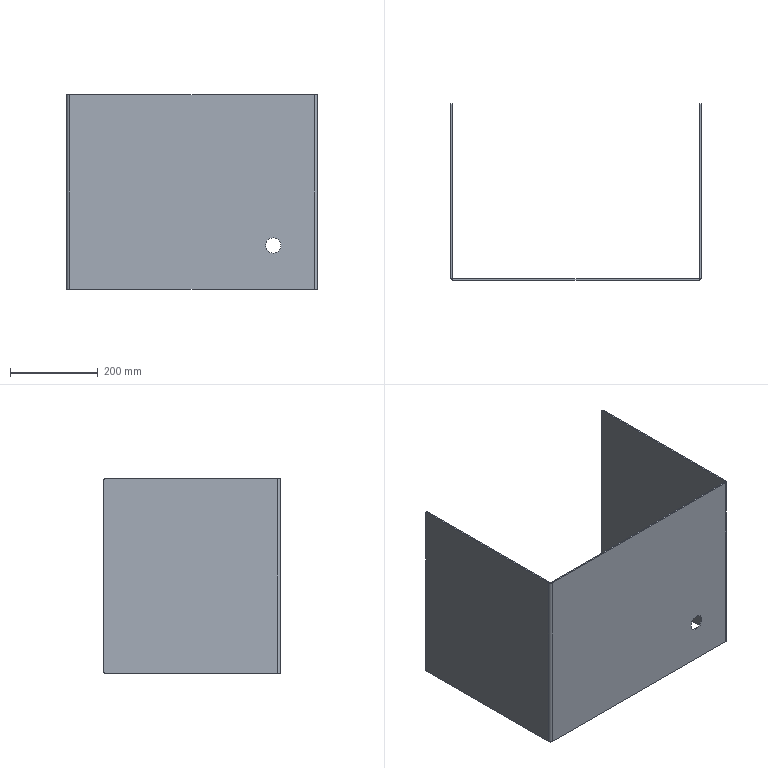Part | SolidWorks | features ICE 2, FlatPattern 1, SMBaseFlange 1, SheetMetal 1 | 1 solid | 28 faces | box 571 x 403 x 444 mm | volume 1818117 mm3 | plane 18 | cylinder 10 | commonest cylinder face diameters 6 x6 12 x2 35 x2
STEP:
#1=CARTESIAN_POINT('',(471.,3.,82.5));
#2=VERTEX_POINT('',#1);
#3=CARTESIAN_POINT('',(471.,3.,117.5));
#4=VERTEX_POINT('',#3);
#5=CARTESIAN_POINT('',(471.,3.,100.));
#6=DIRECTION('',(0.,1.,0.));
#7=DIRECTION('',(0.,0.,1.));
#8=AXIS2_PLACEMENT_3D('',#5,#6,#7);
#9=CIRCLE('',#8,17.5);
#10=EDGE_CURVE('',#2,#4,#9,.T.);
#11=ORIENTED_EDGE('',*,*,#10,.T.);
#12=CARTESIAN_POINT('',(471.,0.,117.5));
#13=VERTEX_POINT('',#12);
#14=CARTESIAN_POINT('',(471.,10.,117.5));
#15=DIRECTION('',(0.,-1.,0.));
#16=VECTOR('',#15,1000.);
#17=LINE('',#14,#16);
#18=EDGE_CURVE('',#4,#13,#17,.T.);
#19=ORIENTED_EDGE('',*,*,#18,.T.);
#20=CARTESIAN_POINT('',(471.,0.,82.5));
#21=VERTEX_POINT('',#20);
#22=CARTESIAN_POINT('',(471.,0.,100.));
#23=DIRECTION('',(0.,-1.,0.));
#24=DIRECTION('',(0.,0.,-1.));
#25=AXIS2_PLACEMENT_3D('',#22,#23,#24);
#26=CIRCLE('',#25,17.5);
#27=EDGE_CURVE('',#13,#21,#26,.T.);
#28=ORIENTED_EDGE('',*,*,#27,.T.);
#29=CARTESIAN_POINT('',(471.,10.,82.5));
#30=DIRECTION('',(0.,-1.,0.));
#31=VECTOR('',#30,1000.);
#32=LINE('',#29,#31);
#33=EDGE_CURVE('',#2,#21,#32,.T.);
#34=ORIENTED_EDGE('',*,*,#33,.F.);
#35=EDGE_LOOP('',(#11,#19,#28,#34));
#36=FACE_OUTER_BOUND('',#35,.T.);
#37=CARTESIAN_POINT('',(471.,10.,100.));
#38=DIRECTION('',(0.,-1.,0.));
#39=DIRECTION('',(0.,0.,-1.));
#40=AXIS2_PLACEMENT_3D('',#37,#38,#39);
#41=CYLINDRICAL_SURFACE('',#40,17.5);
#42=ADVANCED_FACE('',(#36),#41,.F.);
#43=CARTESIAN_POINT('',(571.,400.,0.));
#44=VERTEX_POINT('',#43);
#45=CARTESIAN_POINT('',(571.,403.,3.));
#46=VERTEX_POINT('',#45);
#47=CARTESIAN_POINT('',(571.,400.,3.));
#48=DIRECTION('',(1.,0.,0.));
#49=DIRECTION('',(0.,0.,1.));
#50=AXIS2_PLACEMENT_3D('',#47,#48,#49);
#51=CIRCLE('',#50,3.);
#52=EDGE_CURVE('',#44,#46,#51,.T.);
#53=ORIENTED_EDGE('',*,*,#52,.T.);
#54=CARTESIAN_POINT('',(571.,403.,441.));
#55=VERTEX_POINT('',#54);
#56=CARTESIAN_POINT('',(571.,403.,444.));
#57=DIRECTION('',(0.,0.,-1.));
#58=VECTOR('',#57,1000.);
#59=LINE('',#56,#58);
#60=EDGE_CURVE('',#55,#46,#59,.T.);
#61=ORIENTED_EDGE('',*,*,#60,.F.);
#62=CARTESIAN_POINT('',(571.,400.,444.));
#63=VERTEX_POINT('',#62);
#64=CARTESIAN_POINT('',(571.,400.,441.));
#65=DIRECTION('',(1.,0.,0.));
#66=DIRECTION('',(0.,0.,1.));
#67=AXIS2_PLACEMENT_3D('',#64,#65,#66);
#68=CIRCLE('',#67,3.);
#69=EDGE_CURVE('',#55,#63,#68,.T.);
#70=ORIENTED_EDGE('',*,*,#69,.T.);
#71=CARTESIAN_POINT('',(571.,6.,444.));
#72=VERTEX_POINT('',#71);
#73=CARTESIAN_POINT('',(571.,0.,444.));
#74=DIRECTION('',(0.,1.,0.));
#75=VECTOR('',#74,1000.);
#76=LINE('',#73,#75);
#77=EDGE_CURVE('',#72,#63,#76,.T.);
#78=ORIENTED_EDGE('',*,*,#77,.F.);
#79=CARTESIAN_POINT('',(571.,6.,0.));
#80=VERTEX_POINT('',#79);
#81=CARTESIAN_POINT('',(571.,6.,444.));
#82=DIRECTION('',(0.,0.,-1.));
#83=VECTOR('',#82,1000.);
#84=LINE('',#81,#83);
#85=EDGE_CURVE('',#72,#80,#84,.T.);
#86=ORIENTED_EDGE('',*,*,#85,.T.);
#87=CARTESIAN_POINT('',(571.,0.,0.));
#88=DIRECTION('',(0.,1.,0.));
#89=VECTOR('',#88,1000.);
#90=LINE('',#87,#89);
#91=EDGE_CURVE('',#80,#44,#90,.T.);
#92=ORIENTED_EDGE('',*,*,#91,.T.);
#93=EDGE_LOOP('',(#53,#61,#70,#78,#86,#92));
#94=FACE_OUTER_BOUND('',#93,.T.);
#95=CARTESIAN_POINT('',(571.,0.,444.));
#96=DIRECTION('',(-1.,0.,0.));
#97=DIRECTION('',(0.,0.,1.));
#98=AXIS2_PLACEMENT_3D('',#95,#96,#97);
#99=PLANE('',#98);
#100=ADVANCED_FACE('',(#94),#99,.F.);
#101=CARTESIAN_POINT('',(568.,403.,441.));
#102=VERTEX_POINT('',#101);
#103=CARTESIAN_POINT('',(568.,403.,3.));
#104=VERTEX_POINT('',#103);
#105=CARTESIAN_POINT('',(568.,403.,444.));
#106=DIRECTION('',(0.,0.,-1.));
#107=VECTOR('',#106,1000.);
#108=LINE('',#105,#107);
#109=EDGE_CURVE('',#102,#104,#108,.T.);
#110=ORIENTED_EDGE('',*,*,#109,.T.);
#111=CARTESIAN_POINT('',(568.,400.,0.));
#112=VERTEX_POINT('',#111);
#113=CARTESIAN_POINT('',(568.,400.,3.));
#114=DIRECTION('',(1.,0.,0.));
#115=DIRECTION('',(0.,0.,1.));
#116=AXIS2_PLACEMENT_3D('',#113,#114,#115);
#117=CIRCLE('',#116,3.);
#118=EDGE_CURVE('',#112,#104,#117,.T.);
#119=ORIENTED_EDGE('',*,*,#118,.F.);
#120=CARTESIAN_POINT('',(568.,6.,0.));
#121=VERTEX_POINT('',#120);
#122=CARTESIAN_POINT('',(568.,0.,0.));
#123=DIRECTION('',(0.,1.,0.));
#124=VECTOR('',#123,1000.);
#125=LINE('',#122,#124);
#126=EDGE_CURVE('',#121,#112,#125,.T.);
#127=ORIENTED_EDGE('',*,*,#126,.F.);
#128=CARTESIAN_POINT('',(568.,6.,444.));
#129=VERTEX_POINT('',#128);
#130=CARTESIAN_POINT('',(568.,6.,444.));
#131=DIRECTION('',(0.,0.,-1.));
#132=VECTOR('',#131,1000.);
#133=LINE('',#130,#132);
#134=EDGE_CURVE('',#129,#121,#133,.T.);
#135=ORIENTED_EDGE('',*,*,#134,.F.);
#136=CARTESIAN_POINT('',(568.,400.,444.));
#137=VERTEX_POINT('',#136);
#138=CARTESIAN_POINT('',(568.,0.,444.));
#139=DIRECTION('',(0.,1.,0.));
#140=VECTOR('',#139,1000.);
#141=LINE('',#138,#140);
#142=EDGE_CURVE('',#129,#137,#141,.T.);
#143=ORIENTED_EDGE('',*,*,#142,.T.);
#144=CARTESIAN_POINT('',(568.,400.,441.));
#145=DIRECTION('',(1.,0.,0.));
#146=DIRECTION('',(0.,0.,1.));
#147=AXIS2_PLACEMENT_3D('',#144,#145,#146);
#148=CIRCLE('',#147,3.);
#149=EDGE_CURVE('',#102,#137,#148,.T.);
#150=ORIENTED_EDGE('',*,*,#149,.F.);
#151=EDGE_LOOP('',(#110,#119,#127,#135,#143,#150));
#152=FACE_OUTER_BOUND('',#151,.T.);
#153=CARTESIAN_POINT('',(568.,0.,444.));
#154=DIRECTION('',(-1.,0.,0.));
#155=DIRECTION('',(0.,0.,1.));
#156=AXIS2_PLACEMENT_3D('',#153,#154,#155);
#157=PLANE('',#156);
#158=ADVANCED_FACE('',(#152),#157,.T.);
#159=ORIENTED_EDGE('',*,*,#60,.T.);
#160=CARTESIAN_POINT('',(568.,403.,3.));
#161=DIRECTION('',(1.,0.,0.));
#162=VECTOR('',#161,1000.);
#163=LINE('',#160,#162);
#164=EDGE_CURVE('',#104,#46,#163,.T.);
#165=ORIENTED_EDGE('',*,*,#164,.F.);
#166=ORIENTED_EDGE('',*,*,#109,.F.);
#167=CARTESIAN_POINT('',(568.,403.,441.));
#168=DIRECTION('',(1.,0.,0.));
#169=VECTOR('',#168,1000.);
#170=LINE('',#167,#169);
#171=EDGE_CURVE('',#102,#55,#170,.T.);
#172=ORIENTED_EDGE('',*,*,#171,.T.);
#173=EDGE_LOOP('',(#159,#165,#166,#172));
#174=FACE_OUTER_BOUND('',#173,.T.);
#175=CARTESIAN_POINT('',(568.,403.,444.));
#176=DIRECTION('',(0.,1.,0.));
#177=DIRECTION('',(0.,0.,1.));
#178=AXIS2_PLACEMENT_3D('',#175,#176,#177);
#179=PLANE('',#178);
#180=ADVANCED_FACE('',(#174),#179,.T.);
#181=CARTESIAN_POINT('',(3.,400.,0.));
#182=VERTEX_POINT('',#181);
#183=CARTESIAN_POINT('',(3.,6.,0.));
#184=VERTEX_POINT('',#183);
#185=CARTESIAN_POINT('',(3.,0.,0.));
#186=DIRECTION('',(0.,-1.,0.));
#187=VECTOR('',#186,1000.);
#188=LINE('',#185,#187);
#189=EDGE_CURVE('',#182,#184,#188,.T.);
#190=ORIENTED_EDGE('',*,*,#189,.F.);
#191=CARTESIAN_POINT('',(3.,403.,3.));
#192=VERTEX_POINT('',#191);
#193=CARTESIAN_POINT('',(3.,400.,3.));
#194=DIRECTION('',(-1.,0.,0.));
#195=DIRECTION('',(0.,0.,-1.));
#196=AXIS2_PLACEMENT_3D('',#193,#194,#195);
#197=CIRCLE('',#196,3.);
#198=EDGE_CURVE('',#192,#182,#197,.T.);
#199=ORIENTED_EDGE('',*,*,#198,.F.);
#200=CARTESIAN_POINT('',(3.,403.,441.));
#201=VERTEX_POINT('',#200);
#202=CARTESIAN_POINT('',(3.,403.,444.));
#203=DIRECTION('',(0.,0.,-1.));
#204=VECTOR('',#203,1000.);
#205=LINE('',#202,#204);
#206=EDGE_CURVE('',#201,#192,#205,.T.);
#207=ORIENTED_EDGE('',*,*,#206,.F.);
#208=CARTESIAN_POINT('',(3.,400.,444.));
#209=VERTEX_POINT('',#208);
#210=CARTESIAN_POINT('',(3.,400.,441.));
#211=DIRECTION('',(-1.,0.,0.));
#212=DIRECTION('',(0.,0.,-1.));
#213=AXIS2_PLACEMENT_3D('',#210,#211,#212);
#214=CIRCLE('',#213,3.);
#215=EDGE_CURVE('',#209,#201,#214,.T.);
#216=ORIENTED_EDGE('',*,*,#215,.F.);
#217=CARTESIAN_POINT('',(3.,6.,444.));
#218=VERTEX_POINT('',#217);
#219=CARTESIAN_POINT('',(3.,0.,444.));
#220=DIRECTION('',(0.,-1.,0.));
#221=VECTOR('',#220,1000.);
#222=LINE('',#219,#221);
#223=EDGE_CURVE('',#209,#218,#222,.T.);
#224=ORIENTED_EDGE('',*,*,#223,.T.);
#225=CARTESIAN_POINT('',(3.,6.,444.));
#226=DIRECTION('',(0.,0.,-1.));
#227=VECTOR('',#226,1000.);
#228=LINE('',#225,#227);
#229=EDGE_CURVE('',#218,#184,#228,.T.);
#230=ORIENTED_EDGE('',*,*,#229,.T.);
#231=EDGE_LOOP('',(#190,#199,#207,#216,#224,#230));
#232=FACE_OUTER_BOUND('',#231,.T.);
#233=CARTESIAN_POINT('',(3.,0.,444.));
#234=DIRECTION('',(1.,0.,0.));
#235=DIRECTION('',(0.,0.,-1.));
#236=AXIS2_PLACEMENT_3D('',#233,#234,#235);
#237=PLANE('',#236);
#238=ADVANCED_FACE('',(#232),#237,.T.);
#239=CARTESIAN_POINT('',(0.,403.,3.));
#240=VERTEX_POINT('',#239);
#241=CARTESIAN_POINT('',(0.,400.,0.));
#242=VERTEX_POINT('',#241);
#243=CARTESIAN_POINT('',(0.,400.,3.));
#244=DIRECTION('',(-1.,0.,0.));
#245=DIRECTION('',(0.,0.,-1.));
#246=AXIS2_PLACEMENT_3D('',#243,#244,#245);
#247=CIRCLE('',#246,3.);
#248=EDGE_CURVE('',#240,#242,#247,.T.);
#249=ORIENTED_EDGE('',*,*,#248,.T.);
#250=CARTESIAN_POINT('',(0.,6.,0.));
#251=VERTEX_POINT('',#250);
#252=CARTESIAN_POINT('',(0.,0.,0.));
#253=DIRECTION('',(0.,-1.,0.));
#254=VECTOR('',#253,1000.);
#255=LINE('',#252,#254);
#256=EDGE_CURVE('',#242,#251,#255,.T.);
#257=ORIENTED_EDGE('',*,*,#256,.T.);
#258=CARTESIAN_POINT('',(0.,6.,444.));
#259=VERTEX_POINT('',#258);
#260=CARTESIAN_POINT('',(0.,6.,444.));
#261=DIRECTION('',(0.,0.,-1.));
#262=VECTOR('',#261,1000.);
#263=LINE('',#260,#262);
#264=EDGE_CURVE('',#259,#251,#263,.T.);
#265=ORIENTED_EDGE('',*,*,#264,.F.);
#266=CARTESIAN_POINT('',(0.,400.,444.));
#267=VERTEX_POINT('',#266);
#268=CARTESIAN_POINT('',(0.,0.,444.));
#269=DIRECTION('',(0.,-1.,0.));
#270=VECTOR('',#269,1000.);
#271=LINE('',#268,#270);
#272=EDGE_CURVE('',#267,#259,#271,.T.);
#273=ORIENTED_EDGE('',*,*,#272,.F.);
#274=CARTESIAN_POINT('',(0.,403.,441.));
#275=VERTEX_POINT('',#274);
#276=CARTESIAN_POINT('',(0.,400.,441.));
#277=DIRECTION('',(-1.,0.,0.));
#278=DIRECTION('',(0.,0.,-1.));
#279=AXIS2_PLACEMENT_3D('',#276,#277,#278);
#280=CIRCLE('',#279,3.);
#281=EDGE_CURVE('',#267,#275,#280,.T.);
#282=ORIENTED_EDGE('',*,*,#281,.T.);
#283=CARTESIAN_POINT('',(0.,403.,444.));
#284=DIRECTION('',(0.,0.,-1.));
#285=VECTOR('',#284,1000.);
#286=LINE('',#283,#285);
#287=EDGE_CURVE('',#275,#240,#286,.T.);
#288=ORIENTED_EDGE('',*,*,#287,.T.);
#289=EDGE_LOOP('',(#249,#257,#265,#273,#282,#288));
#290=FACE_OUTER_BOUND('',#289,.T.);
#291=CARTESIAN_POINT('',(0.,0.,444.));
#292=DIRECTION('',(1.,0.,0.));
#293=DIRECTION('',(0.,0.,-1.));
#294=AXIS2_PLACEMENT_3D('',#291,#292,#293);
#295=PLANE('',#294);
#296=ADVANCED_FACE('',(#290),#295,.F.);
#297=ORIENTED_EDGE('',*,*,#77,.T.);
#298=CARTESIAN_POINT('',(568.,400.,444.));
#299=DIRECTION('',(1.,0.,0.));
#300=VECTOR('',#299,1000.);
#301=LINE('',#298,#300);
#302=EDGE_CURVE('',#137,#63,#301,.T.);
#303=ORIENTED_EDGE('',*,*,#302,.F.);
#304=ORIENTED_EDGE('',*,*,#142,.F.);
#305=CARTESIAN_POINT('',(568.,6.,444.));
#306=DIRECTION('',(1.,0.,0.));
#307=VECTOR('',#306,1000.);
#308=LINE('',#305,#307);
#309=EDGE_CURVE('',#129,#72,#308,.T.);
#310=ORIENTED_EDGE('',*,*,#309,.T.);
#311=EDGE_LOOP('',(#297,#303,#304,#310));
#312=FACE_OUTER_BOUND('',#311,.T.);
#313=CARTESIAN_POINT('',(565.,6.,444.));
#314=DIRECTION('',(0.,0.,1.));
#315=DIRECTION('',(1.,0.,0.));
#316=AXIS2_PLACEMENT_3D('',#313,#314,#315);
#317=PLANE('',#316);
#318=ADVANCED_FACE('',(#312),#317,.T.);
#319=CARTESIAN_POINT('',(3.,403.,3.));
#320=DIRECTION('',(-1.,0.,0.));
#321=VECTOR('',#320,1000.);
#322=LINE('',#319,#321);
#323=EDGE_CURVE('',#192,#240,#322,.T.);
#324=ORIENTED_EDGE('',*,*,#323,.T.);
#325=ORIENTED_EDGE('',*,*,#287,.F.);
#326=CARTESIAN_POINT('',(3.,403.,441.));
#327=DIRECTION('',(-1.,0.,0.));
#328=VECTOR('',#327,1000.);
#329=LINE('',#326,#328);
#330=EDGE_CURVE('',#201,#275,#329,.T.);
#331=ORIENTED_EDGE('',*,*,#330,.F.);
#332=ORIENTED_EDGE('',*,*,#206,.T.);
#333=EDGE_LOOP('',(#324,#325,#331,#332));
#334=FACE_OUTER_BOUND('',#333,.T.);
#335=CARTESIAN_POINT('',(0.,403.,444.));
#336=DIRECTION('',(0.,1.,0.));
#337=DIRECTION('',(0.,0.,1.));
#338=AXIS2_PLACEMENT_3D('',#335,#336,#337);
#339=PLANE('',#338);
#340=ADVANCED_FACE('',(#334),#339,.T.);
#341=CARTESIAN_POINT('',(0.,6.,444.));
#342=DIRECTION('',(1.,0.,0.));
#343=VECTOR('',#342,1000.);
#344=LINE('',#341,#343);
#345=EDGE_CURVE('',#259,#218,#344,.T.);
#346=ORIENTED_EDGE('',*,*,#345,.F.);
#347=CARTESIAN_POINT('',(6.,0.,444.));
#348=VERTEX_POINT('',#347);
#349=CARTESIAN_POINT('',(6.,6.,444.));
#350=DIRECTION('',(0.,0.,1.));
#351=DIRECTION('',(-1.,0.,0.));
#352=AXIS2_PLACEMENT_3D('',#349,#350,#351);
#353=CIRCLE('',#352,6.);
#354=EDGE_CURVE('',#259,#348,#353,.T.);
#355=ORIENTED_EDGE('',*,*,#354,.T.);
#356=CARTESIAN_POINT('',(6.,3.,444.));
#357=VERTEX_POINT('',#356);
#358=CARTESIAN_POINT('',(6.,3.,444.));
#359=DIRECTION('',(0.,-1.,0.));
#360=VECTOR('',#359,1000.);
#361=LINE('',#358,#360);
#362=EDGE_CURVE('',#357,#348,#361,.T.);
#363=ORIENTED_EDGE('',*,*,#362,.F.);
#364=CARTESIAN_POINT('',(6.,6.,444.));
#365=DIRECTION('',(0.,0.,1.));
#366=DIRECTION('',(1.,0.,0.));
#367=AXIS2_PLACEMENT_3D('',#364,#365,#366);
#368=CIRCLE('',#367,3.);
#369=EDGE_CURVE('',#218,#357,#368,.T.);
#370=ORIENTED_EDGE('',*,*,#369,.F.);
#371=EDGE_LOOP('',(#346,#355,#363,#370));
#372=FACE_OUTER_BOUND('',#371,.T.);
#373=CARTESIAN_POINT('',(0.,6.,444.));
#374=DIRECTION('',(0.,0.,1.));
#375=DIRECTION('',(1.,0.,0.));
#376=AXIS2_PLACEMENT_3D('',#373,#374,#375);
#377=PLANE('',#376);
#378=ADVANCED_FACE('',(#372),#377,.T.);
#379=CARTESIAN_POINT('',(3.,400.,444.));
#380=DIRECTION('',(-1.,0.,0.));
#381=VECTOR('',#380,1000.);
#382=LINE('',#379,#381);
#383=EDGE_CURVE('',#209,#267,#382,.T.);
#384=ORIENTED_EDGE('',*,*,#383,.T.);
#385=ORIENTED_EDGE('',*,*,#272,.T.);
#386=ORIENTED_EDGE('',*,*,#345,.T.);
#387=ORIENTED_EDGE('',*,*,#223,.F.);
#388=EDGE_LOOP('',(#384,#385,#386,#387));
#389=FACE_OUTER_BOUND('',#388,.T.);
#390=CARTESIAN_POINT('',(6.,3.,444.));
#391=DIRECTION('',(0.,0.,1.));
#392=DIRECTION('',(1.,0.,0.));
#393=AXIS2_PLACEMENT_3D('',#390,#391,#392);
#394=PLANE('',#393);
#395=ADVANCED_FACE('',(#389),#394,.T.);
#396=CARTESIAN_POINT('',(6.,0.,0.));
#397=VERTEX_POINT('',#396);
#398=CARTESIAN_POINT('',(6.,3.,0.));
#399=VERTEX_POINT('',#398);
#400=CARTESIAN_POINT('',(6.,0.,0.));
#401=DIRECTION('',(0.,1.,0.));
#402=VECTOR('',#401,1000.);
#403=LINE('',#400,#402);
#404=EDGE_CURVE('',#397,#399,#403,.T.);
#405=ORIENTED_EDGE('',*,*,#404,.F.);
#406=CARTESIAN_POINT('',(6.,6.,0.));
#407=DIRECTION('',(0.,0.,1.));
#408=DIRECTION('',(-1.,0.,0.));
#409=AXIS2_PLACEMENT_3D('',#406,#407,#408);
#410=CIRCLE('',#409,6.);
#411=EDGE_CURVE('',#251,#397,#410,.T.);
#412=ORIENTED_EDGE('',*,*,#411,.F.);
#413=CARTESIAN_POINT('',(3.,6.,0.));
#414=DIRECTION('',(-1.,0.,0.));
#415=VECTOR('',#414,1000.);
#416=LINE('',#413,#415);
#417=EDGE_CURVE('',#184,#251,#416,.T.);
#418=ORIENTED_EDGE('',*,*,#417,.F.);
#419=CARTESIAN_POINT('',(6.,6.,0.));
#420=DIRECTION('',(0.,0.,1.));
#421=DIRECTION('',(1.,0.,0.));
#422=AXIS2_PLACEMENT_3D('',#419,#420,#421);
#423=CIRCLE('',#422,3.);
#424=EDGE_CURVE('',#184,#399,#423,.T.);
#425=ORIENTED_EDGE('',*,*,#424,.T.);
#426=EDGE_LOOP('',(#405,#412,#418,#425));
#427=FACE_OUTER_BOUND('',#426,.T.);
#428=CARTESIAN_POINT('',(6.,0.,0.));
#429=DIRECTION('',(0.,0.,-1.));
#430=DIRECTION('',(-1.,0.,0.));
#431=AXIS2_PLACEMENT_3D('',#428,#429,#430);
#432=PLANE('',#431);
#433=ADVANCED_FACE('',(#427),#432,.T.);
#434=CARTESIAN_POINT('',(565.,0.,0.));
#435=VERTEX_POINT('',#434);
#436=CARTESIAN_POINT('',(0.,0.,0.));
#437=DIRECTION('',(1.,0.,0.));
#438=VECTOR('',#437,1000.);
#439=LINE('',#436,#438);
#440=EDGE_CURVE('',#397,#435,#439,.T.);
#441=ORIENTED_EDGE('',*,*,#440,.F.);
#442=ORIENTED_EDGE('',*,*,#404,.T.);
#443=CARTESIAN_POINT('',(565.,3.,0.));
#444=VERTEX_POINT('',#443);
#445=CARTESIAN_POINT('',(0.,3.,0.));
#446=DIRECTION('',(1.,0.,0.));
#447=VECTOR('',#446,1000.);
#448=LINE('',#445,#447);
#449=EDGE_CURVE('',#399,#444,#448,.T.);
#450=ORIENTED_EDGE('',*,*,#449,.T.);
#451=CARTESIAN_POINT('',(565.,3.,0.));
#452=DIRECTION('',(0.,-1.,0.));
#453=VECTOR('',#452,1000.);
#454=LINE('',#451,#453);
#455=EDGE_CURVE('',#444,#435,#454,.T.);
#456=ORIENTED_EDGE('',*,*,#455,.T.);
#457=EDGE_LOOP('',(#441,#442,#450,#456));
#458=FACE_OUTER_BOUND('',#457,.T.);
#459=CARTESIAN_POINT('',(3.,6.,0.));
#460=DIRECTION('',(0.,0.,-1.));
#461=DIRECTION('',(-1.,0.,0.));
#462=AXIS2_PLACEMENT_3D('',#459,#460,#461);
#463=PLANE('',#462);
#464=ADVANCED_FACE('',(#458),#463,.T.);
#465=CARTESIAN_POINT('',(565.,0.,444.));
#466=VERTEX_POINT('',#465);
#467=CARTESIAN_POINT('',(565.,3.,444.));
#468=VERTEX_POINT('',#467);
#469=CARTESIAN_POINT('',(565.,0.,444.));
#470=DIRECTION('',(0.,1.,0.));
#471=VECTOR('',#470,1000.);
#472=LINE('',#469,#471);
#473=EDGE_CURVE('',#466,#468,#472,.T.);
#474=ORIENTED_EDGE('',*,*,#473,.F.);
#475=CARTESIAN_POINT('',(565.,6.,444.));
#476=DIRECTION('',(0.,0.,1.));
#477=DIRECTION('',(-1.,0.,0.));
#478=AXIS2_PLACEMENT_3D('',#475,#476,#477);
#479=CIRCLE('',#478,6.);
#480=EDGE_CURVE('',#466,#72,#479,.T.);
#481=ORIENTED_EDGE('',*,*,#480,.T.);
#482=ORIENTED_EDGE('',*,*,#309,.F.);
#483=CARTESIAN_POINT('',(565.,6.,444.));
#484=DIRECTION('',(0.,0.,1.));
#485=DIRECTION('',(1.,0.,0.));
#486=AXIS2_PLACEMENT_3D('',#483,#484,#485);
#487=CIRCLE('',#486,3.);
#488=EDGE_CURVE('',#468,#129,#487,.T.);
#489=ORIENTED_EDGE('',*,*,#488,.F.);
#490=EDGE_LOOP('',(#474,#481,#482,#489));
#491=FACE_OUTER_BOUND('',#490,.T.);
#492=CARTESIAN_POINT('',(565.,0.,444.));
#493=DIRECTION('',(0.,0.,1.));
#494=DIRECTION('',(1.,0.,0.));
#495=AXIS2_PLACEMENT_3D('',#492,#493,#494);
#496=PLANE('',#495);
#497=ADVANCED_FACE('',(#491),#496,.T.);
#498=CARTESIAN_POINT('',(0.,0.,444.));
#499=DIRECTION('',(1.,0.,0.));
#500=VECTOR('',#499,1000.);
#501=LINE('',#498,#500);
#502=EDGE_CURVE('',#348,#466,#501,.T.);
#503=ORIENTED_EDGE('',*,*,#502,.T.);
#504=ORIENTED_EDGE('',*,*,#473,.T.);
#505=CARTESIAN_POINT('',(0.,3.,444.));
#506=DIRECTION('',(1.,0.,0.));
#507=VECTOR('',#506,1000.);
#508=LINE('',#505,#507);
#509=EDGE_CURVE('',#357,#468,#508,.T.);
#510=ORIENTED_EDGE('',*,*,#509,.F.);
#511=ORIENTED_EDGE('',*,*,#362,.T.);
#512=EDGE_LOOP('',(#503,#504,#510,#511));
#513=FACE_OUTER_BOUND('',#512,.T.);
#514=CARTESIAN_POINT('',(568.,6.,444.));
#515=DIRECTION('',(0.,0.,1.));
#516=DIRECTION('',(1.,0.,0.));
#517=AXIS2_PLACEMENT_3D('',#514,#515,#516);
#518=PLANE('',#517);
#519=ADVANCED_FACE('',(#513),#518,.T.);
#520=CARTESIAN_POINT('',(571.,6.,0.));
#521=DIRECTION('',(-1.,0.,0.));
#522=VECTOR('',#521,1000.);
#523=LINE('',#520,#522);
#524=EDGE_CURVE('',#80,#121,#523,.T.);
#525=ORIENTED_EDGE('',*,*,#524,.F.);
#526=CARTESIAN_POINT('',(565.,6.,0.));
#527=DIRECTION('',(0.,0.,1.));
#528=DIRECTION('',(-1.,0.,0.));
#529=AXIS2_PLACEMENT_3D('',#526,#527,#528);
#530=CIRCLE('',#529,6.);
#531=EDGE_CURVE('',#435,#80,#530,.T.);
#532=ORIENTED_EDGE('',*,*,#531,.F.);
#533=ORIENTED_EDGE('',*,*,#455,.F.);
#534=CARTESIAN_POINT('',(565.,6.,0.));
#535=DIRECTION('',(0.,0.,1.));
#536=DIRECTION('',(1.,0.,0.));
#537=AXIS2_PLACEMENT_3D('',#534,#535,#536);
#538=CIRCLE('',#537,3.);
#539=EDGE_CURVE('',#444,#121,#538,.T.);
#540=ORIENTED_EDGE('',*,*,#539,.T.);
#541=EDGE_LOOP('',(#525,#532,#533,#540));
#542=FACE_OUTER_BOUND('',#541,.T.);
#543=CARTESIAN_POINT('',(571.,6.,0.));
#544=DIRECTION('',(0.,0.,-1.));
#545=DIRECTION('',(-1.,0.,0.));
#546=AXIS2_PLACEMENT_3D('',#543,#544,#545);
#547=PLANE('',#546);
#548=ADVANCED_FACE('',(#542),#547,.T.);
#549=CARTESIAN_POINT('',(568.,400.,0.));
#550=DIRECTION('',(1.,0.,0.));
#551=VECTOR('',#550,1000.);
#552=LINE('',#549,#551);
#553=EDGE_CURVE('',#112,#44,#552,.T.);
#554=ORIENTED_EDGE('',*,*,#553,.T.);
#555=ORIENTED_EDGE('',*,*,#91,.F.);
#556=ORIENTED_EDGE('',*,*,#524,.T.);
#557=ORIENTED_EDGE('',*,*,#126,.T.);
#558=EDGE_LOOP('',(#554,#555,#556,#557));
#559=FACE_OUTER_BOUND('',#558,.T.);
#560=CARTESIAN_POINT('',(565.,3.,0.));
#561=DIRECTION('',(0.,0.,-1.));
#562=DIRECTION('',(-1.,0.,0.));
#563=AXIS2_PLACEMENT_3D('',#560,#561,#562);
#564=PLANE('',#563);
#565=ADVANCED_FACE('',(#559),#564,.T.);
#566=ORIENTED_EDGE('',*,*,#539,.F.);
#567=CARTESIAN_POINT('',(565.,3.,444.));
#568=DIRECTION('',(0.,0.,-1.));
#569=VECTOR('',#568,1000.);
#570=LINE('',#567,#569);
#571=EDGE_CURVE('',#468,#444,#570,.T.);
#572=ORIENTED_EDGE('',*,*,#571,.F.);
#573=ORIENTED_EDGE('',*,*,#488,.T.);
#574=ORIENTED_EDGE('',*,*,#134,.T.);
#575=EDGE_LOOP('',(#566,#572,#573,#574));
#576=FACE_OUTER_BOUND('',#575,.T.);
#577=CARTESIAN_POINT('',(565.,6.,444.));
#578=DIRECTION('',(0.,0.,-1.));
#579=DIRECTION('',(-1.,0.,0.));
#580=AXIS2_PLACEMENT_3D('',#577,#578,#579);
#581=CYLINDRICAL_SURFACE('',#580,3.);
#582=ADVANCED_FACE('',(#576),#581,.F.);
#583=ORIENTED_EDGE('',*,*,#10,.F.);
#584=CARTESIAN_POINT('',(471.,3.,100.));
#585=DIRECTION('',(0.,1.,0.));
#586=DIRECTION('',(0.,0.,1.));
#587=AXIS2_PLACEMENT_3D('',#584,#585,#586);
#588=CIRCLE('',#587,17.5);
#589=EDGE_CURVE('',#4,#2,#588,.T.);
#590=ORIENTED_EDGE('',*,*,#589,.F.);
#591=EDGE_LOOP('',(#583,#590));
#592=FACE_BOUND('',#591,.T.);
#593=ORIENTED_EDGE('',*,*,#449,.F.);
#594=CARTESIAN_POINT('',(6.,3.,444.));
#595=DIRECTION('',(0.,0.,-1.));
#596=VECTOR('',#595,1000.);
#597=LINE('',#594,#596);
#598=EDGE_CURVE('',#357,#399,#597,.T.);
#599=ORIENTED_EDGE('',*,*,#598,.F.);
#600=ORIENTED_EDGE('',*,*,#509,.T.);
#601=ORIENTED_EDGE('',*,*,#571,.T.);
#602=EDGE_LOOP('',(#593,#599,#600,#601));
#603=FACE_OUTER_BOUND('',#602,.T.);
#604=CARTESIAN_POINT('',(0.,3.,444.));
#605=DIRECTION('',(0.,1.,0.));
#606=DIRECTION('',(0.,0.,1.));
#607=AXIS2_PLACEMENT_3D('',#604,#605,#606);
#608=PLANE('',#607);
#609=ADVANCED_FACE('',(#592,#603),#608,.T.);
#610=ORIENTED_EDGE('',*,*,#424,.F.);
#611=ORIENTED_EDGE('',*,*,#229,.F.);
#612=ORIENTED_EDGE('',*,*,#369,.T.);
#613=ORIENTED_EDGE('',*,*,#598,.T.);
#614=EDGE_LOOP('',(#610,#611,#612,#613));
#615=FACE_OUTER_BOUND('',#614,.T.);
#616=CARTESIAN_POINT('',(6.,6.,444.));
#617=DIRECTION('',(0.,0.,-1.));
#618=DIRECTION('',(-1.,0.,0.));
#619=AXIS2_PLACEMENT_3D('',#616,#617,#618);
#620=CYLINDRICAL_SURFACE('',#619,3.);
#621=ADVANCED_FACE('',(#615),#620,.F.);
#622=ORIENTED_EDGE('',*,*,#411,.T.);
#623=CARTESIAN_POINT('',(6.,0.,444.));
#624=DIRECTION('',(0.,0.,-1.));
#625=VECTOR('',#624,1000.);
#626=LINE('',#623,#625);
#627=EDGE_CURVE('',#348,#397,#626,.T.);
#628=ORIENTED_EDGE('',*,*,#627,.F.);
#629=ORIENTED_EDGE('',*,*,#354,.F.);
#630=ORIENTED_EDGE('',*,*,#264,.T.);
#631=EDGE_LOOP('',(#622,#628,#629,#630));
#632=FACE_OUTER_BOUND('',#631,.T.);
#633=CARTESIAN_POINT('',(6.,6.,444.));
#634=DIRECTION('',(0.,0.,-1.));
#635=DIRECTION('',(-1.,0.,0.));
#636=AXIS2_PLACEMENT_3D('',#633,#634,#635);
#637=CYLINDRICAL_SURFACE('',#636,6.);
#638=ADVANCED_FACE('',(#632),#637,.T.);
#639=CARTESIAN_POINT('',(471.,0.,100.));
#640=DIRECTION('',(0.,-1.,0.));
#641=DIRECTION('',(0.,0.,-1.));
#642=AXIS2_PLACEMENT_3D('',#639,#640,#641);
#643=CIRCLE('',#642,17.5);
#644=EDGE_CURVE('',#21,#13,#643,.T.);
#645=ORIENTED_EDGE('',*,*,#644,.F.);
#646=ORIENTED_EDGE('',*,*,#27,.F.);
#647=EDGE_LOOP('',(#645,#646));
#648=FACE_BOUND('',#647,.T.);
#649=ORIENTED_EDGE('',*,*,#440,.T.);
#650=CARTESIAN_POINT('',(565.,0.,444.));
#651=DIRECTION('',(0.,0.,-1.));
#652=VECTOR('',#651,1000.);
#653=LINE('',#650,#652);
#654=EDGE_CURVE('',#466,#435,#653,.T.);
#655=ORIENTED_EDGE('',*,*,#654,.F.);
#656=ORIENTED_EDGE('',*,*,#502,.F.);
#657=ORIENTED_EDGE('',*,*,#627,.T.);
#658=EDGE_LOOP('',(#649,#655,#656,#657));
#659=FACE_OUTER_BOUND('',#658,.T.);
#660=CARTESIAN_POINT('',(0.,0.,444.));
#661=DIRECTION('',(0.,1.,0.));
#662=DIRECTION('',(0.,0.,1.));
#663=AXIS2_PLACEMENT_3D('',#660,#661,#662);
#664=PLANE('',#663);
#665=ADVANCED_FACE('',(#648,#659),#664,.F.);
#666=ORIENTED_EDGE('',*,*,#531,.T.);
#667=ORIENTED_EDGE('',*,*,#85,.F.);
#668=ORIENTED_EDGE('',*,*,#480,.F.);
#669=ORIENTED_EDGE('',*,*,#654,.T.);
#670=EDGE_LOOP('',(#666,#667,#668,#669));
#671=FACE_OUTER_BOUND('',#670,.T.);
#672=CARTESIAN_POINT('',(565.,6.,444.));
#673=DIRECTION('',(0.,0.,-1.));
#674=DIRECTION('',(-1.,0.,0.));
#675=AXIS2_PLACEMENT_3D('',#672,#673,#674);
#676=CYLINDRICAL_SURFACE('',#675,6.);
#677=ADVANCED_FACE('',(#671),#676,.T.);
#678=ORIENTED_EDGE('',*,*,#256,.F.);
#679=CARTESIAN_POINT('',(3.,400.,0.));
#680=DIRECTION('',(-1.,0.,0.));
#681=VECTOR('',#680,1000.);
#682=LINE('',#679,#681);
#683=EDGE_CURVE('',#182,#242,#682,.T.);
#684=ORIENTED_EDGE('',*,*,#683,.F.);
#685=ORIENTED_EDGE('',*,*,#189,.T.);
#686=ORIENTED_EDGE('',*,*,#417,.T.);
#687=EDGE_LOOP('',(#678,#684,#685,#686));
#688=FACE_OUTER_BOUND('',#687,.T.);
#689=CARTESIAN_POINT('',(565.,6.,0.));
#690=DIRECTION('',(0.,0.,1.));
#691=DIRECTION('',(1.,0.,0.));
#692=AXIS2_PLACEMENT_3D('',#689,#690,#691);
#693=PLANE('',#692);
#694=ADVANCED_FACE('',(#688),#693,.F.);
#695=ORIENTED_EDGE('',*,*,#18,.F.);
#696=ORIENTED_EDGE('',*,*,#589,.T.);
#697=ORIENTED_EDGE('',*,*,#33,.T.);
#698=ORIENTED_EDGE('',*,*,#644,.T.);
#699=EDGE_LOOP('',(#695,#696,#697,#698));
#700=FACE_OUTER_BOUND('',#699,.T.);
#701=CARTESIAN_POINT('',(471.,10.,100.));
#702=DIRECTION('',(0.,-1.,0.));
#703=DIRECTION('',(0.,0.,-1.));
#704=AXIS2_PLACEMENT_3D('',#701,#702,#703);
#705=CYLINDRICAL_SURFACE('',#704,17.5);
#706=ADVANCED_FACE('',(#700),#705,.F.);
#707=ORIENTED_EDGE('',*,*,#215,.T.);
#708=ORIENTED_EDGE('',*,*,#330,.T.);
#709=ORIENTED_EDGE('',*,*,#281,.F.);
#710=ORIENTED_EDGE('',*,*,#383,.F.);
#711=EDGE_LOOP('',(#707,#708,#709,#710));
#712=FACE_OUTER_BOUND('',#711,.T.);
#713=CARTESIAN_POINT('',(3.,400.,441.));
#714=DIRECTION('',(1.,0.,0.));
#715=DIRECTION('',(0.,0.,-1.));
#716=AXIS2_PLACEMENT_3D('',#713,#714,#715);
#717=CYLINDRICAL_SURFACE('',#716,3.);
#718=ADVANCED_FACE('',(#712),#717,.T.);
#719=ORIENTED_EDGE('',*,*,#149,.T.);
#720=ORIENTED_EDGE('',*,*,#302,.T.);
#721=ORIENTED_EDGE('',*,*,#69,.F.);
#722=ORIENTED_EDGE('',*,*,#171,.F.);
#723=EDGE_LOOP('',(#719,#720,#721,#722));
#724=FACE_OUTER_BOUND('',#723,.T.);
#725=CARTESIAN_POINT('',(568.,400.,441.));
#726=DIRECTION('',(-1.,0.,0.));
#727=DIRECTION('',(0.,0.,1.));
#728=AXIS2_PLACEMENT_3D('',#725,#726,#727);
#729=CYLINDRICAL_SURFACE('',#728,3.);
#730=ADVANCED_FACE('',(#724),#729,.T.);
#731=ORIENTED_EDGE('',*,*,#198,.T.);
#732=ORIENTED_EDGE('',*,*,#683,.T.);
#733=ORIENTED_EDGE('',*,*,#248,.F.);
#734=ORIENTED_EDGE('',*,*,#323,.F.);
#735=EDGE_LOOP('',(#731,#732,#733,#734));
#736=FACE_OUTER_BOUND('',#735,.T.);
#737=CARTESIAN_POINT('',(3.,400.,3.));
#738=DIRECTION('',(1.,0.,0.));
#739=DIRECTION('',(0.,0.,-1.));
#740=AXIS2_PLACEMENT_3D('',#737,#738,#739);
#741=CYLINDRICAL_SURFACE('',#740,3.);
#742=ADVANCED_FACE('',(#736),#741,.T.);
#743=ORIENTED_EDGE('',*,*,#118,.T.);
#744=ORIENTED_EDGE('',*,*,#164,.T.);
#745=ORIENTED_EDGE('',*,*,#52,.F.);
#746=ORIENTED_EDGE('',*,*,#553,.F.);
#747=EDGE_LOOP('',(#743,#744,#745,#746));
#748=FACE_OUTER_BOUND('',#747,.T.);
#749=CARTESIAN_POINT('',(568.,400.,3.));
#750=DIRECTION('',(-1.,0.,0.));
#751=DIRECTION('',(0.,0.,1.));
#752=AXIS2_PLACEMENT_3D('',#749,#750,#751);
#753=CYLINDRICAL_SURFACE('',#752,3.);
#754=ADVANCED_FACE('',(#748),#753,.T.);
#755=CLOSED_SHELL('',(#42,#100,#158,#180,#238,#296,#318,#340,#378,#395,#433,#464,#497,#519,#548,#565,#582,#609,#621,#638,#665,#677,#694,#706,#718,#730,#742,#754));
#756=MANIFOLD_SOLID_BREP('',#755);
#757=CARTESIAN_POINT('',(0.,0.,0.));
#758=DIRECTION('',(0.,0.,1.));
#759=DIRECTION('',(1.,0.,0.));
#760=AXIS2_PLACEMENT_3D('',#757,#758,#759);
#761=(LENGTH_UNIT()NAMED_UNIT(*)SI_UNIT(.MILLI.,.METRE.));
#762=UNCERTAINTY_MEASURE_WITH_UNIT(LENGTH_MEASURE(0.00001),#761,'','');
#763=(NAMED_UNIT(*)PLANE_ANGLE_UNIT()SI_UNIT($,.RADIAN.));
#764=(NAMED_UNIT(*)SI_UNIT($,.STERADIAN.)SOLID_ANGLE_UNIT());
#765=(GEOMETRIC_REPRESENTATION_CONTEXT(3)GLOBAL_UNCERTAINTY_ASSIGNED_CONTEXT((#762))GLOBAL_UNIT_ASSIGNED_CONTEXT((#761,#763,#764))REPRESENTATION_CONTEXT('',''));
#766=ADVANCED_BREP_SHAPE_REPRESENTATION('',(#756,#760),#765);